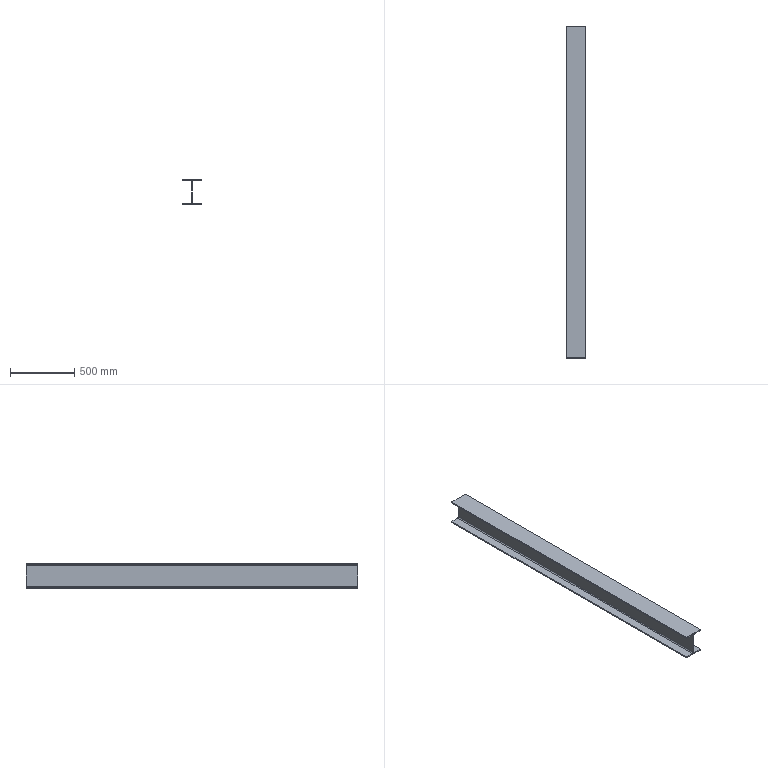Part | STEP file | Metering column 5 body_Default<As Machined> | 1 solid | 18 faces | box 150 x 2578 x 194 mm | volume 9824598 mm3 | plane 14 | cylinder 4 | commonest cylinder face diameters 16 x4
STEP:
#1=CARTESIAN_POINT('',(0.,0.,0.));
#2=DIRECTION('',(0.,0.,1.));
#3=DIRECTION('',(1.,0.,0.));
#4=AXIS2_PLACEMENT_3D('',#1,#2,#3);
#5=CARTESIAN_POINT('',(75.,0.,-88.));
#6=VERTEX_POINT('',#5);
#7=CARTESIAN_POINT('',(75.,0.,-97.));
#8=VERTEX_POINT('',#7);
#9=CARTESIAN_POINT('',(75.,0.,-97.));
#10=DIRECTION('',(0.,0.,-1.));
#11=VECTOR('',#10,1.);
#12=LINE('',#9,#11);
#13=CARTESIAN_POINT('',(75.,2578.,-97.));
#14=DIRECTION('',(-1.,0.,0.));
#15=DIRECTION('',(0.,0.,1.));
#16=AXIS2_PLACEMENT_3D('',#13,#14,#15);
#17=PLANE('',#16);
#18=CARTESIAN_POINT('',(0.,-2578.));
#19=DIRECTION('',(-1.,0.));
#20=VECTOR('',#19,1.);
#21=LINE('',#18,#20);
#22=(GEOMETRIC_REPRESENTATION_CONTEXT(2)PARAMETRIC_REPRESENTATION_CONTEXT()REPRESENTATION_CONTEXT('',''));
#23=DEFINITIONAL_REPRESENTATION('',(#21),#22);
#24=PCURVE('',#17,#23);
#25=CARTESIAN_POINT('',(11.,0.,-80.));
#26=DIRECTION('',(0.,1.,0.));
#27=DIRECTION('',(0.,0.,1.));
#28=AXIS2_PLACEMENT_3D('',#25,#26,#27);
#29=PLANE('',#28);
#30=CARTESIAN_POINT('',(-17.,64.));
#31=DIRECTION('',(-1.,0.));
#32=VECTOR('',#31,1.);
#33=LINE('',#30,#32);
#34=(GEOMETRIC_REPRESENTATION_CONTEXT(2)PARAMETRIC_REPRESENTATION_CONTEXT()REPRESENTATION_CONTEXT('',''));
#35=DEFINITIONAL_REPRESENTATION('',(#33),#34);
#36=PCURVE('',#29,#35);
#37=SURFACE_CURVE('',#12,(#24,#36),.PCURVE_S1.);
#38=EDGE_CURVE('',#6,#8,#37,.T.);
#39=ORIENTED_EDGE('',*,*,#38,.T.);
#40=CARTESIAN_POINT('',(75.,2578.,-97.));
#41=VERTEX_POINT('',#40);
#42=CARTESIAN_POINT('',(75.,2578.,-97.));
#43=DIRECTION('',(0.,-1.,0.));
#44=VECTOR('',#43,1.);
#45=LINE('',#42,#44);
#46=CARTESIAN_POINT('',(0.,0.));
#47=DIRECTION('',(0.,-1.));
#48=VECTOR('',#47,1.);
#49=LINE('',#46,#48);
#50=(GEOMETRIC_REPRESENTATION_CONTEXT(2)PARAMETRIC_REPRESENTATION_CONTEXT()REPRESENTATION_CONTEXT('',''));
#51=DEFINITIONAL_REPRESENTATION('',(#49),#50);
#52=PCURVE('',#17,#51);
#53=CARTESIAN_POINT('',(75.,2578.,-97.));
#54=DIRECTION('',(0.,0.,1.));
#55=DIRECTION('',(1.,0.,0.));
#56=AXIS2_PLACEMENT_3D('',#53,#54,#55);
#57=PLANE('',#56);
#58=CARTESIAN_POINT('',(0.,0.));
#59=DIRECTION('',(0.,-1.));
#60=VECTOR('',#59,1.);
#61=LINE('',#58,#60);
#62=(GEOMETRIC_REPRESENTATION_CONTEXT(2)PARAMETRIC_REPRESENTATION_CONTEXT()REPRESENTATION_CONTEXT('',''));
#63=DEFINITIONAL_REPRESENTATION('',(#61),#62);
#64=PCURVE('',#57,#63);
#65=SURFACE_CURVE('',#45,(#52,#64),.PCURVE_S1.);
#66=EDGE_CURVE('',#41,#8,#65,.T.);
#67=ORIENTED_EDGE('',*,*,#66,.F.);
#68=CARTESIAN_POINT('',(75.,2578.,-88.));
#69=VERTEX_POINT('',#68);
#70=CARTESIAN_POINT('',(75.,2578.,-97.));
#71=DIRECTION('',(0.,0.,-1.));
#72=VECTOR('',#71,1.);
#73=LINE('',#70,#72);
#74=CARTESIAN_POINT('',(0.,0.));
#75=DIRECTION('',(-1.,0.));
#76=VECTOR('',#75,1.);
#77=LINE('',#74,#76);
#78=(GEOMETRIC_REPRESENTATION_CONTEXT(2)PARAMETRIC_REPRESENTATION_CONTEXT()REPRESENTATION_CONTEXT('',''));
#79=DEFINITIONAL_REPRESENTATION('',(#77),#78);
#80=PCURVE('',#17,#79);
#81=CARTESIAN_POINT('',(11.,2578.,-80.));
#82=DIRECTION('',(0.,1.,0.));
#83=DIRECTION('',(0.,0.,1.));
#84=AXIS2_PLACEMENT_3D('',#81,#82,#83);
#85=PLANE('',#84);
#86=CARTESIAN_POINT('',(-17.,64.));
#87=DIRECTION('',(-1.,0.));
#88=VECTOR('',#87,1.);
#89=LINE('',#86,#88);
#90=(GEOMETRIC_REPRESENTATION_CONTEXT(2)PARAMETRIC_REPRESENTATION_CONTEXT()REPRESENTATION_CONTEXT('',''));
#91=DEFINITIONAL_REPRESENTATION('',(#89),#90);
#92=PCURVE('',#85,#91);
#93=SURFACE_CURVE('',#73,(#80,#92),.PCURVE_S1.);
#94=EDGE_CURVE('',#69,#41,#93,.T.);
#95=ORIENTED_EDGE('',*,*,#94,.F.);
#96=CARTESIAN_POINT('',(75.,2578.,-88.));
#97=DIRECTION('',(0.,-1.,0.));
#98=VECTOR('',#97,1.);
#99=LINE('',#96,#98);
#100=CARTESIAN_POINT('',(9.,0.));
#101=DIRECTION('',(0.,-1.));
#102=VECTOR('',#101,1.);
#103=LINE('',#100,#102);
#104=(GEOMETRIC_REPRESENTATION_CONTEXT(2)PARAMETRIC_REPRESENTATION_CONTEXT()REPRESENTATION_CONTEXT('',''));
#105=DEFINITIONAL_REPRESENTATION('',(#103),#104);
#106=PCURVE('',#17,#105);
#107=CARTESIAN_POINT('',(75.,2578.,-88.));
#108=DIRECTION('',(0.,0.,-1.));
#109=DIRECTION('',(-1.,0.,0.));
#110=AXIS2_PLACEMENT_3D('',#107,#108,#109);
#111=PLANE('',#110);
#112=CARTESIAN_POINT('',(0.,0.));
#113=DIRECTION('',(0.,-1.));
#114=VECTOR('',#113,1.);
#115=LINE('',#112,#114);
#116=(GEOMETRIC_REPRESENTATION_CONTEXT(2)PARAMETRIC_REPRESENTATION_CONTEXT()REPRESENTATION_CONTEXT('',''));
#117=DEFINITIONAL_REPRESENTATION('',(#115),#116);
#118=PCURVE('',#111,#117);
#119=SURFACE_CURVE('',#99,(#106,#118),.PCURVE_S1.);
#120=EDGE_CURVE('',#69,#6,#119,.T.);
#121=ORIENTED_EDGE('',*,*,#120,.T.);
#122=EDGE_LOOP('',(#39,#67,#95,#121));
#123=FACE_BOUND('',#122,.T.);
#124=ADVANCED_FACE('',(#123),#17,.F.);
#125=CARTESIAN_POINT('',(-75.,0.,-97.));
#126=VERTEX_POINT('',#125);
#127=CARTESIAN_POINT('',(75.,0.,-97.));
#128=DIRECTION('',(-1.,0.,0.));
#129=VECTOR('',#128,1.);
#130=LINE('',#127,#129);
#131=CARTESIAN_POINT('',(0.,-2578.));
#132=DIRECTION('',(-1.,0.));
#133=VECTOR('',#132,1.);
#134=LINE('',#131,#133);
#135=(GEOMETRIC_REPRESENTATION_CONTEXT(2)PARAMETRIC_REPRESENTATION_CONTEXT()REPRESENTATION_CONTEXT('',''));
#136=DEFINITIONAL_REPRESENTATION('',(#134),#135);
#137=PCURVE('',#57,#136);
#138=CARTESIAN_POINT('',(-17.,64.));
#139=DIRECTION('',(0.,-1.));
#140=VECTOR('',#139,1.);
#141=LINE('',#138,#140);
#142=(GEOMETRIC_REPRESENTATION_CONTEXT(2)PARAMETRIC_REPRESENTATION_CONTEXT()REPRESENTATION_CONTEXT('',''));
#143=DEFINITIONAL_REPRESENTATION('',(#141),#142);
#144=PCURVE('',#29,#143);
#145=SURFACE_CURVE('',#130,(#137,#144),.PCURVE_S1.);
#146=EDGE_CURVE('',#8,#126,#145,.T.);
#147=ORIENTED_EDGE('',*,*,#146,.T.);
#148=CARTESIAN_POINT('',(-75.,2578.,-97.));
#149=VERTEX_POINT('',#148);
#150=CARTESIAN_POINT('',(-75.,2578.,-97.));
#151=DIRECTION('',(0.,-1.,0.));
#152=VECTOR('',#151,1.);
#153=LINE('',#150,#152);
#154=CARTESIAN_POINT('',(-150.,0.));
#155=DIRECTION('',(0.,-1.));
#156=VECTOR('',#155,1.);
#157=LINE('',#154,#156);
#158=(GEOMETRIC_REPRESENTATION_CONTEXT(2)PARAMETRIC_REPRESENTATION_CONTEXT()REPRESENTATION_CONTEXT('',''));
#159=DEFINITIONAL_REPRESENTATION('',(#157),#158);
#160=PCURVE('',#57,#159);
#161=CARTESIAN_POINT('',(-75.,2578.,-88.));
#162=DIRECTION('',(1.,0.,0.));
#163=DIRECTION('',(0.,0.,-1.));
#164=AXIS2_PLACEMENT_3D('',#161,#162,#163);
#165=PLANE('',#164);
#166=CARTESIAN_POINT('',(9.,0.));
#167=DIRECTION('',(0.,-1.));
#168=VECTOR('',#167,1.);
#169=LINE('',#166,#168);
#170=(GEOMETRIC_REPRESENTATION_CONTEXT(2)PARAMETRIC_REPRESENTATION_CONTEXT()REPRESENTATION_CONTEXT('',''));
#171=DEFINITIONAL_REPRESENTATION('',(#169),#170);
#172=PCURVE('',#165,#171);
#173=SURFACE_CURVE('',#153,(#160,#172),.PCURVE_S1.);
#174=EDGE_CURVE('',#149,#126,#173,.T.);
#175=ORIENTED_EDGE('',*,*,#174,.F.);
#176=CARTESIAN_POINT('',(75.,2578.,-97.));
#177=DIRECTION('',(-1.,0.,0.));
#178=VECTOR('',#177,1.);
#179=LINE('',#176,#178);
#180=CARTESIAN_POINT('',(0.,0.));
#181=DIRECTION('',(-1.,0.));
#182=VECTOR('',#181,1.);
#183=LINE('',#180,#182);
#184=(GEOMETRIC_REPRESENTATION_CONTEXT(2)PARAMETRIC_REPRESENTATION_CONTEXT()REPRESENTATION_CONTEXT('',''));
#185=DEFINITIONAL_REPRESENTATION('',(#183),#184);
#186=PCURVE('',#57,#185);
#187=CARTESIAN_POINT('',(-17.,64.));
#188=DIRECTION('',(0.,-1.));
#189=VECTOR('',#188,1.);
#190=LINE('',#187,#189);
#191=(GEOMETRIC_REPRESENTATION_CONTEXT(2)PARAMETRIC_REPRESENTATION_CONTEXT()REPRESENTATION_CONTEXT('',''));
#192=DEFINITIONAL_REPRESENTATION('',(#190),#191);
#193=PCURVE('',#85,#192);
#194=SURFACE_CURVE('',#179,(#186,#193),.PCURVE_S1.);
#195=EDGE_CURVE('',#41,#149,#194,.T.);
#196=ORIENTED_EDGE('',*,*,#195,.F.);
#197=ORIENTED_EDGE('',*,*,#66,.T.);
#198=EDGE_LOOP('',(#147,#175,#196,#197));
#199=FACE_BOUND('',#198,.T.);
#200=ADVANCED_FACE('',(#199),#57,.F.);
#201=CARTESIAN_POINT('',(-75.,0.,-88.));
#202=VERTEX_POINT('',#201);
#203=CARTESIAN_POINT('',(-75.,0.,-88.));
#204=DIRECTION('',(0.,0.,1.));
#205=VECTOR('',#204,1.);
#206=LINE('',#203,#205);
#207=CARTESIAN_POINT('',(0.,-2578.));
#208=DIRECTION('',(-1.,0.));
#209=VECTOR('',#208,1.);
#210=LINE('',#207,#209);
#211=(GEOMETRIC_REPRESENTATION_CONTEXT(2)PARAMETRIC_REPRESENTATION_CONTEXT()REPRESENTATION_CONTEXT('',''));
#212=DEFINITIONAL_REPRESENTATION('',(#210),#211);
#213=PCURVE('',#165,#212);
#214=CARTESIAN_POINT('',(-8.,-86.));
#215=DIRECTION('',(1.,0.));
#216=VECTOR('',#215,1.);
#217=LINE('',#214,#216);
#218=(GEOMETRIC_REPRESENTATION_CONTEXT(2)PARAMETRIC_REPRESENTATION_CONTEXT()REPRESENTATION_CONTEXT('',''));
#219=DEFINITIONAL_REPRESENTATION('',(#217),#218);
#220=PCURVE('',#29,#219);
#221=SURFACE_CURVE('',#206,(#213,#220),.PCURVE_S1.);
#222=EDGE_CURVE('',#126,#202,#221,.T.);
#223=ORIENTED_EDGE('',*,*,#222,.T.);
#224=CARTESIAN_POINT('',(-75.,2578.,-88.));
#225=VERTEX_POINT('',#224);
#226=CARTESIAN_POINT('',(-75.,2578.,-88.));
#227=DIRECTION('',(0.,-1.,0.));
#228=VECTOR('',#227,1.);
#229=LINE('',#226,#228);
#230=CARTESIAN_POINT('',(0.,0.));
#231=DIRECTION('',(0.,-1.));
#232=VECTOR('',#231,1.);
#233=LINE('',#230,#232);
#234=(GEOMETRIC_REPRESENTATION_CONTEXT(2)PARAMETRIC_REPRESENTATION_CONTEXT()REPRESENTATION_CONTEXT('',''));
#235=DEFINITIONAL_REPRESENTATION('',(#233),#234);
#236=PCURVE('',#165,#235);
#237=CARTESIAN_POINT('',(-11.,2578.,-88.));
#238=DIRECTION('',(0.,0.,-1.));
#239=DIRECTION('',(-1.,0.,0.));
#240=AXIS2_PLACEMENT_3D('',#237,#238,#239);
#241=PLANE('',#240);
#242=CARTESIAN_POINT('',(64.,0.));
#243=DIRECTION('',(0.,-1.));
#244=VECTOR('',#243,1.);
#245=LINE('',#242,#244);
#246=(GEOMETRIC_REPRESENTATION_CONTEXT(2)PARAMETRIC_REPRESENTATION_CONTEXT()REPRESENTATION_CONTEXT('',''));
#247=DEFINITIONAL_REPRESENTATION('',(#245),#246);
#248=PCURVE('',#241,#247);
#249=SURFACE_CURVE('',#229,(#236,#248),.PCURVE_S1.);
#250=EDGE_CURVE('',#225,#202,#249,.T.);
#251=ORIENTED_EDGE('',*,*,#250,.F.);
#252=CARTESIAN_POINT('',(-75.,2578.,-88.));
#253=DIRECTION('',(0.,0.,1.));
#254=VECTOR('',#253,1.);
#255=LINE('',#252,#254);
#256=CARTESIAN_POINT('',(0.,0.));
#257=DIRECTION('',(-1.,0.));
#258=VECTOR('',#257,1.);
#259=LINE('',#256,#258);
#260=(GEOMETRIC_REPRESENTATION_CONTEXT(2)PARAMETRIC_REPRESENTATION_CONTEXT()REPRESENTATION_CONTEXT('',''));
#261=DEFINITIONAL_REPRESENTATION('',(#259),#260);
#262=PCURVE('',#165,#261);
#263=CARTESIAN_POINT('',(-8.,-86.));
#264=DIRECTION('',(1.,0.));
#265=VECTOR('',#264,1.);
#266=LINE('',#263,#265);
#267=(GEOMETRIC_REPRESENTATION_CONTEXT(2)PARAMETRIC_REPRESENTATION_CONTEXT()REPRESENTATION_CONTEXT('',''));
#268=DEFINITIONAL_REPRESENTATION('',(#266),#267);
#269=PCURVE('',#85,#268);
#270=SURFACE_CURVE('',#255,(#262,#269),.PCURVE_S1.);
#271=EDGE_CURVE('',#149,#225,#270,.T.);
#272=ORIENTED_EDGE('',*,*,#271,.F.);
#273=ORIENTED_EDGE('',*,*,#174,.T.);
#274=EDGE_LOOP('',(#223,#251,#272,#273));
#275=FACE_BOUND('',#274,.T.);
#276=ADVANCED_FACE('',(#275),#165,.F.);
#277=CARTESIAN_POINT('',(-11.,0.,-88.));
#278=VERTEX_POINT('',#277);
#279=CARTESIAN_POINT('',(-11.,0.,-88.));
#280=DIRECTION('',(1.,0.,0.));
#281=VECTOR('',#280,1.);
#282=LINE('',#279,#281);
#283=CARTESIAN_POINT('',(0.,-2578.));
#284=DIRECTION('',(-1.,0.));
#285=VECTOR('',#284,1.);
#286=LINE('',#283,#285);
#287=(GEOMETRIC_REPRESENTATION_CONTEXT(2)PARAMETRIC_REPRESENTATION_CONTEXT()REPRESENTATION_CONTEXT('',''));
#288=DEFINITIONAL_REPRESENTATION('',(#286),#287);
#289=PCURVE('',#241,#288);
#290=CARTESIAN_POINT('',(-8.,-22.));
#291=DIRECTION('',(0.,1.));
#292=VECTOR('',#291,1.);
#293=LINE('',#290,#292);
#294=(GEOMETRIC_REPRESENTATION_CONTEXT(2)PARAMETRIC_REPRESENTATION_CONTEXT()REPRESENTATION_CONTEXT('',''));
#295=DEFINITIONAL_REPRESENTATION('',(#293),#294);
#296=PCURVE('',#29,#295);
#297=SURFACE_CURVE('',#282,(#289,#296),.PCURVE_S1.);
#298=EDGE_CURVE('',#202,#278,#297,.T.);
#299=ORIENTED_EDGE('',*,*,#298,.T.);
#300=CARTESIAN_POINT('',(-11.,2578.,-88.));
#301=VERTEX_POINT('',#300);
#302=CARTESIAN_POINT('',(-11.,2578.,-88.));
#303=DIRECTION('',(0.,-1.,0.));
#304=VECTOR('',#303,1.);
#305=LINE('',#302,#304);
#306=CARTESIAN_POINT('',(0.,0.));
#307=DIRECTION('',(0.,-1.));
#308=VECTOR('',#307,1.);
#309=LINE('',#306,#308);
#310=(GEOMETRIC_REPRESENTATION_CONTEXT(2)PARAMETRIC_REPRESENTATION_CONTEXT()REPRESENTATION_CONTEXT('',''));
#311=DEFINITIONAL_REPRESENTATION('',(#309),#310);
#312=PCURVE('',#241,#311);
#313=CARTESIAN_POINT('',(-11.,2578.,-80.));
#314=DIRECTION('',(0.,-1.,0.));
#315=DIRECTION('',(0.,0.,-1.));
#316=AXIS2_PLACEMENT_3D('',#313,#314,#315);
#317=CYLINDRICAL_SURFACE('',#316,8.);
#318=CARTESIAN_POINT('',(0.,0.));
#319=DIRECTION('',(0.,1.));
#320=VECTOR('',#319,1.);
#321=LINE('',#318,#320);
#322=(GEOMETRIC_REPRESENTATION_CONTEXT(2)PARAMETRIC_REPRESENTATION_CONTEXT()REPRESENTATION_CONTEXT('',''));
#323=DEFINITIONAL_REPRESENTATION('',(#321),#322);
#324=PCURVE('',#317,#323);
#325=SURFACE_CURVE('',#305,(#312,#324),.PCURVE_S1.);
#326=EDGE_CURVE('',#301,#278,#325,.T.);
#327=ORIENTED_EDGE('',*,*,#326,.F.);
#328=CARTESIAN_POINT('',(-11.,2578.,-88.));
#329=DIRECTION('',(1.,0.,0.));
#330=VECTOR('',#329,1.);
#331=LINE('',#328,#330);
#332=CARTESIAN_POINT('',(0.,0.));
#333=DIRECTION('',(-1.,0.));
#334=VECTOR('',#333,1.);
#335=LINE('',#332,#334);
#336=(GEOMETRIC_REPRESENTATION_CONTEXT(2)PARAMETRIC_REPRESENTATION_CONTEXT()REPRESENTATION_CONTEXT('',''));
#337=DEFINITIONAL_REPRESENTATION('',(#335),#336);
#338=PCURVE('',#241,#337);
#339=CARTESIAN_POINT('',(-8.,-22.));
#340=DIRECTION('',(0.,1.));
#341=VECTOR('',#340,1.);
#342=LINE('',#339,#341);
#343=(GEOMETRIC_REPRESENTATION_CONTEXT(2)PARAMETRIC_REPRESENTATION_CONTEXT()REPRESENTATION_CONTEXT('',''));
#344=DEFINITIONAL_REPRESENTATION('',(#342),#343);
#345=PCURVE('',#85,#344);
#346=SURFACE_CURVE('',#331,(#338,#345),.PCURVE_S1.);
#347=EDGE_CURVE('',#225,#301,#346,.T.);
#348=ORIENTED_EDGE('',*,*,#347,.F.);
#349=ORIENTED_EDGE('',*,*,#250,.T.);
#350=EDGE_LOOP('',(#299,#327,#348,#349));
#351=FACE_BOUND('',#350,.T.);
#352=ADVANCED_FACE('',(#351),#241,.F.);
#353=ORIENTED_EDGE('',*,*,#326,.F.);
#354=CARTESIAN_POINT('',(-3.,2578.,-80.));
#355=VERTEX_POINT('',#354);
#356=CARTESIAN_POINT('',(-11.,2578.,-80.));
#357=DIRECTION('',(0.,-1.,0.));
#358=DIRECTION('',(0.,0.,1.));
#359=AXIS2_PLACEMENT_3D('',#356,#357,#358);
#360=CIRCLE('',#359,8.);
#361=CARTESIAN_POINT('',(-3.142,0.));
#362=DIRECTION('',(1.,0.));
#363=VECTOR('',#362,1.);
#364=LINE('',#361,#363);
#365=(GEOMETRIC_REPRESENTATION_CONTEXT(2)PARAMETRIC_REPRESENTATION_CONTEXT()REPRESENTATION_CONTEXT('',''));
#366=DEFINITIONAL_REPRESENTATION('',(#364),#365);
#367=PCURVE('',#317,#366);
#368=CARTESIAN_POINT('',(8.,-22.));
#369=CARTESIAN_POINT('',(8.,-35.856));
#370=CARTESIAN_POINT('',(-4.,-28.928));
#371=CARTESIAN_POINT('',(-16.,-22.));
#372=CARTESIAN_POINT('',(-4.,-15.072));
#373=CARTESIAN_POINT('',(8.,-8.144));
#374=CARTESIAN_POINT('',(8.,-22.));
#375=(BOUNDED_CURVE()B_SPLINE_CURVE(2,(#368,#369,#370,#371,#372,#373,#374),.UNSPECIFIED.,.T.,.F.)B_SPLINE_CURVE_WITH_KNOTS((1,2,2,2,2,1),(-2.094,0.,2.094,4.189,6.283,8.378),.UNSPECIFIED.)CURVE()GEOMETRIC_REPRESENTATION_ITEM()RATIONAL_B_SPLINE_CURVE((1.,0.5,1.,0.5,1.,0.5,1.))REPRESENTATION_ITEM(''));
#376=(GEOMETRIC_REPRESENTATION_CONTEXT(2)PARAMETRIC_REPRESENTATION_CONTEXT()REPRESENTATION_CONTEXT('',''));
#377=DEFINITIONAL_REPRESENTATION('',(#375),#376);
#378=PCURVE('',#85,#377);
#379=SURFACE_CURVE('',#360,(#367,#378),.PCURVE_S1.);
#380=EDGE_CURVE('',#301,#355,#379,.T.);
#381=ORIENTED_EDGE('',*,*,#380,.T.);
#382=CARTESIAN_POINT('',(-3.,0.,-80.));
#383=VERTEX_POINT('',#382);
#384=CARTESIAN_POINT('',(-3.,2578.,-80.));
#385=DIRECTION('',(0.,-1.,0.));
#386=VECTOR('',#385,1.);
#387=LINE('',#384,#386);
#388=CARTESIAN_POINT('',(1.571,0.));
#389=DIRECTION('',(0.,1.));
#390=VECTOR('',#389,1.);
#391=LINE('',#388,#390);
#392=(GEOMETRIC_REPRESENTATION_CONTEXT(2)PARAMETRIC_REPRESENTATION_CONTEXT()REPRESENTATION_CONTEXT('',''));
#393=DEFINITIONAL_REPRESENTATION('',(#391),#392);
#394=PCURVE('',#317,#393);
#395=CARTESIAN_POINT('',(-3.,2578.,80.));
#396=DIRECTION('',(1.,0.,0.));
#397=DIRECTION('',(0.,0.,-1.));
#398=AXIS2_PLACEMENT_3D('',#395,#396,#397);
#399=PLANE('',#398);
#400=CARTESIAN_POINT('',(160.,0.));
#401=DIRECTION('',(0.,-1.));
#402=VECTOR('',#401,1.);
#403=LINE('',#400,#402);
#404=(GEOMETRIC_REPRESENTATION_CONTEXT(2)PARAMETRIC_REPRESENTATION_CONTEXT()REPRESENTATION_CONTEXT('',''));
#405=DEFINITIONAL_REPRESENTATION('',(#403),#404);
#406=PCURVE('',#399,#405);
#407=SURFACE_CURVE('',#387,(#394,#406),.PCURVE_S1.);
#408=EDGE_CURVE('',#355,#383,#407,.T.);
#409=ORIENTED_EDGE('',*,*,#408,.T.);
#410=CARTESIAN_POINT('',(-11.,0.,-80.));
#411=DIRECTION('',(0.,-1.,0.));
#412=DIRECTION('',(0.,0.,1.));
#413=AXIS2_PLACEMENT_3D('',#410,#411,#412);
#414=CIRCLE('',#413,8.);
#415=CARTESIAN_POINT('',(-3.142,2578.));
#416=DIRECTION('',(1.,0.));
#417=VECTOR('',#416,1.);
#418=LINE('',#415,#417);
#419=(GEOMETRIC_REPRESENTATION_CONTEXT(2)PARAMETRIC_REPRESENTATION_CONTEXT()REPRESENTATION_CONTEXT('',''));
#420=DEFINITIONAL_REPRESENTATION('',(#418),#419);
#421=PCURVE('',#317,#420);
#422=CARTESIAN_POINT('',(8.,-22.));
#423=CARTESIAN_POINT('',(8.,-35.856));
#424=CARTESIAN_POINT('',(-4.,-28.928));
#425=CARTESIAN_POINT('',(-16.,-22.));
#426=CARTESIAN_POINT('',(-4.,-15.072));
#427=CARTESIAN_POINT('',(8.,-8.144));
#428=CARTESIAN_POINT('',(8.,-22.));
#429=(BOUNDED_CURVE()B_SPLINE_CURVE(2,(#422,#423,#424,#425,#426,#427,#428),.UNSPECIFIED.,.T.,.F.)B_SPLINE_CURVE_WITH_KNOTS((1,2,2,2,2,1),(-2.094,0.,2.094,4.189,6.283,8.378),.UNSPECIFIED.)CURVE()GEOMETRIC_REPRESENTATION_ITEM()RATIONAL_B_SPLINE_CURVE((1.,0.5,1.,0.5,1.,0.5,1.))REPRESENTATION_ITEM(''));
#430=(GEOMETRIC_REPRESENTATION_CONTEXT(2)PARAMETRIC_REPRESENTATION_CONTEXT()REPRESENTATION_CONTEXT('',''));
#431=DEFINITIONAL_REPRESENTATION('',(#429),#430);
#432=PCURVE('',#29,#431);
#433=SURFACE_CURVE('',#414,(#421,#432),.PCURVE_S1.);
#434=EDGE_CURVE('',#278,#383,#433,.T.);
#435=ORIENTED_EDGE('',*,*,#434,.F.);
#436=EDGE_LOOP('',(#353,#381,#409,#435));
#437=FACE_BOUND('',#436,.F.);
#438=ADVANCED_FACE('',(#437),#317,.F.);
#439=CARTESIAN_POINT('',(-3.,0.,80.));
#440=VERTEX_POINT('',#439);
#441=CARTESIAN_POINT('',(-3.,0.,80.));
#442=DIRECTION('',(0.,0.,1.));
#443=VECTOR('',#442,1.);
#444=LINE('',#441,#443);
#445=CARTESIAN_POINT('',(0.,-2578.));
#446=DIRECTION('',(-1.,0.));
#447=VECTOR('',#446,1.);
#448=LINE('',#445,#447);
#449=(GEOMETRIC_REPRESENTATION_CONTEXT(2)PARAMETRIC_REPRESENTATION_CONTEXT()REPRESENTATION_CONTEXT('',''));
#450=DEFINITIONAL_REPRESENTATION('',(#448),#449);
#451=PCURVE('',#399,#450);
#452=CARTESIAN_POINT('',(160.,-14.));
#453=DIRECTION('',(1.,0.));
#454=VECTOR('',#453,1.);
#455=LINE('',#452,#454);
#456=(GEOMETRIC_REPRESENTATION_CONTEXT(2)PARAMETRIC_REPRESENTATION_CONTEXT()REPRESENTATION_CONTEXT('',''));
#457=DEFINITIONAL_REPRESENTATION('',(#455),#456);
#458=PCURVE('',#29,#457);
#459=SURFACE_CURVE('',#444,(#451,#458),.PCURVE_S1.);
#460=EDGE_CURVE('',#383,#440,#459,.T.);
#461=ORIENTED_EDGE('',*,*,#460,.T.);
#462=CARTESIAN_POINT('',(-3.,2578.,80.));
#463=VERTEX_POINT('',#462);
#464=CARTESIAN_POINT('',(-3.,2578.,80.));
#465=DIRECTION('',(0.,-1.,0.));
#466=VECTOR('',#465,1.);
#467=LINE('',#464,#466);
#468=CARTESIAN_POINT('',(0.,0.));
#469=DIRECTION('',(0.,-1.));
#470=VECTOR('',#469,1.);
#471=LINE('',#468,#470);
#472=(GEOMETRIC_REPRESENTATION_CONTEXT(2)PARAMETRIC_REPRESENTATION_CONTEXT()REPRESENTATION_CONTEXT('',''));
#473=DEFINITIONAL_REPRESENTATION('',(#471),#472);
#474=PCURVE('',#399,#473);
#475=CARTESIAN_POINT('',(-11.,2578.,80.));
#476=DIRECTION('',(0.,-1.,0.));
#477=DIRECTION('',(0.,0.,-1.));
#478=AXIS2_PLACEMENT_3D('',#475,#476,#477);
#479=CYLINDRICAL_SURFACE('',#478,8.);
#480=CARTESIAN_POINT('',(1.571,0.));
#481=DIRECTION('',(0.,1.));
#482=VECTOR('',#481,1.);
#483=LINE('',#480,#482);
#484=(GEOMETRIC_REPRESENTATION_CONTEXT(2)PARAMETRIC_REPRESENTATION_CONTEXT()REPRESENTATION_CONTEXT('',''));
#485=DEFINITIONAL_REPRESENTATION('',(#483),#484);
#486=PCURVE('',#479,#485);
#487=SURFACE_CURVE('',#467,(#474,#486),.PCURVE_S1.);
#488=EDGE_CURVE('',#463,#440,#487,.T.);
#489=ORIENTED_EDGE('',*,*,#488,.F.);
#490=CARTESIAN_POINT('',(-3.,2578.,80.));
#491=DIRECTION('',(0.,0.,1.));
#492=VECTOR('',#491,1.);
#493=LINE('',#490,#492);
#494=CARTESIAN_POINT('',(0.,0.));
#495=DIRECTION('',(-1.,0.));
#496=VECTOR('',#495,1.);
#497=LINE('',#494,#496);
#498=(GEOMETRIC_REPRESENTATION_CONTEXT(2)PARAMETRIC_REPRESENTATION_CONTEXT()REPRESENTATION_CONTEXT('',''));
#499=DEFINITIONAL_REPRESENTATION('',(#497),#498);
#500=PCURVE('',#399,#499);
#501=CARTESIAN_POINT('',(160.,-14.));
#502=DIRECTION('',(1.,0.));
#503=VECTOR('',#502,1.);
#504=LINE('',#501,#503);
#505=(GEOMETRIC_REPRESENTATION_CONTEXT(2)PARAMETRIC_REPRESENTATION_CONTEXT()REPRESENTATION_CONTEXT('',''));
#506=DEFINITIONAL_REPRESENTATION('',(#504),#505);
#507=PCURVE('',#85,#506);
#508=SURFACE_CURVE('',#493,(#500,#507),.PCURVE_S1.);
#509=EDGE_CURVE('',#355,#463,#508,.T.);
#510=ORIENTED_EDGE('',*,*,#509,.F.);
#511=ORIENTED_EDGE('',*,*,#408,.T.);
#512=EDGE_LOOP('',(#461,#489,#510,#511));
#513=FACE_BOUND('',#512,.T.);
#514=ADVANCED_FACE('',(#513),#399,.F.);
#515=ORIENTED_EDGE('',*,*,#488,.F.);
#516=CARTESIAN_POINT('',(-11.,2578.,88.));
#517=VERTEX_POINT('',#516);
#518=CARTESIAN_POINT('',(-11.,2578.,80.));
#519=DIRECTION('',(0.,-1.,0.));
#520=DIRECTION('',(0.,0.,1.));
#521=AXIS2_PLACEMENT_3D('',#518,#519,#520);
#522=CIRCLE('',#521,8.);
#523=CARTESIAN_POINT('',(-3.142,0.));
#524=DIRECTION('',(1.,0.));
#525=VECTOR('',#524,1.);
#526=LINE('',#523,#525);
#527=(GEOMETRIC_REPRESENTATION_CONTEXT(2)PARAMETRIC_REPRESENTATION_CONTEXT()REPRESENTATION_CONTEXT('',''));
#528=DEFINITIONAL_REPRESENTATION('',(#526),#527);
#529=PCURVE('',#479,#528);
#530=CARTESIAN_POINT('',(168.,-22.));
#531=CARTESIAN_POINT('',(168.,-35.856));
#532=CARTESIAN_POINT('',(156.,-28.928));
#533=CARTESIAN_POINT('',(144.,-22.));
#534=CARTESIAN_POINT('',(156.,-15.072));
#535=CARTESIAN_POINT('',(168.,-8.144));
#536=CARTESIAN_POINT('',(168.,-22.));
#537=(BOUNDED_CURVE()B_SPLINE_CURVE(2,(#530,#531,#532,#533,#534,#535,#536),.UNSPECIFIED.,.T.,.F.)B_SPLINE_CURVE_WITH_KNOTS((1,2,2,2,2,1),(-2.094,0.,2.094,4.189,6.283,8.378),.UNSPECIFIED.)CURVE()GEOMETRIC_REPRESENTATION_ITEM()RATIONAL_B_SPLINE_CURVE((1.,0.5,1.,0.5,1.,0.5,1.))REPRESENTATION_ITEM(''));
#538=(GEOMETRIC_REPRESENTATION_CONTEXT(2)PARAMETRIC_REPRESENTATION_CONTEXT()REPRESENTATION_CONTEXT('',''));
#539=DEFINITIONAL_REPRESENTATION('',(#537),#538);
#540=PCURVE('',#85,#539);
#541=SURFACE_CURVE('',#522,(#529,#540),.PCURVE_S1.);
#542=EDGE_CURVE('',#463,#517,#541,.T.);
#543=ORIENTED_EDGE('',*,*,#542,.T.);
#544=CARTESIAN_POINT('',(-11.,0.,88.));
#545=VERTEX_POINT('',#544);
#546=CARTESIAN_POINT('',(-11.,2578.,88.));
#547=DIRECTION('',(0.,-1.,0.));
#548=VECTOR('',#547,1.);
#549=LINE('',#546,#548);
#550=CARTESIAN_POINT('',(3.142,0.));
#551=DIRECTION('',(0.,1.));
#552=VECTOR('',#551,1.);
#553=LINE('',#550,#552);
#554=(GEOMETRIC_REPRESENTATION_CONTEXT(2)PARAMETRIC_REPRESENTATION_CONTEXT()REPRESENTATION_CONTEXT('',''));
#555=DEFINITIONAL_REPRESENTATION('',(#553),#554);
#556=PCURVE('',#479,#555);
#557=CARTESIAN_POINT('',(-75.,2578.,88.));
#558=DIRECTION('',(0.,0.,1.));
#559=DIRECTION('',(1.,0.,0.));
#560=AXIS2_PLACEMENT_3D('',#557,#558,#559);
#561=PLANE('',#560);
#562=CARTESIAN_POINT('',(64.,0.));
#563=DIRECTION('',(0.,-1.));
#564=VECTOR('',#563,1.);
#565=LINE('',#562,#564);
#566=(GEOMETRIC_REPRESENTATION_CONTEXT(2)PARAMETRIC_REPRESENTATION_CONTEXT()REPRESENTATION_CONTEXT('',''));
#567=DEFINITIONAL_REPRESENTATION('',(#565),#566);
#568=PCURVE('',#561,#567);
#569=SURFACE_CURVE('',#549,(#556,#568),.PCURVE_S1.);
#570=EDGE_CURVE('',#517,#545,#569,.T.);
#571=ORIENTED_EDGE('',*,*,#570,.T.);
#572=CARTESIAN_POINT('',(-11.,0.,80.));
#573=DIRECTION('',(0.,-1.,0.));
#574=DIRECTION('',(0.,0.,1.));
#575=AXIS2_PLACEMENT_3D('',#572,#573,#574);
#576=CIRCLE('',#575,8.);
#577=CARTESIAN_POINT('',(-3.142,2578.));
#578=DIRECTION('',(1.,0.));
#579=VECTOR('',#578,1.);
#580=LINE('',#577,#579);
#581=(GEOMETRIC_REPRESENTATION_CONTEXT(2)PARAMETRIC_REPRESENTATION_CONTEXT()REPRESENTATION_CONTEXT('',''));
#582=DEFINITIONAL_REPRESENTATION('',(#580),#581);
#583=PCURVE('',#479,#582);
#584=CARTESIAN_POINT('',(168.,-22.));
#585=CARTESIAN_POINT('',(168.,-35.856));
#586=CARTESIAN_POINT('',(156.,-28.928));
#587=CARTESIAN_POINT('',(144.,-22.));
#588=CARTESIAN_POINT('',(156.,-15.072));
#589=CARTESIAN_POINT('',(168.,-8.144));
#590=CARTESIAN_POINT('',(168.,-22.));
#591=(BOUNDED_CURVE()B_SPLINE_CURVE(2,(#584,#585,#586,#587,#588,#589,#590),.UNSPECIFIED.,.T.,.F.)B_SPLINE_CURVE_WITH_KNOTS((1,2,2,2,2,1),(-2.094,0.,2.094,4.189,6.283,8.378),.UNSPECIFIED.)CURVE()GEOMETRIC_REPRESENTATION_ITEM()RATIONAL_B_SPLINE_CURVE((1.,0.5,1.,0.5,1.,0.5,1.))REPRESENTATION_ITEM(''));
#592=(GEOMETRIC_REPRESENTATION_CONTEXT(2)PARAMETRIC_REPRESENTATION_CONTEXT()REPRESENTATION_CONTEXT('',''));
#593=DEFINITIONAL_REPRESENTATION('',(#591),#592);
#594=PCURVE('',#29,#593);
#595=SURFACE_CURVE('',#576,(#583,#594),.PCURVE_S1.);
#596=EDGE_CURVE('',#440,#545,#595,.T.);
#597=ORIENTED_EDGE('',*,*,#596,.F.);
#598=EDGE_LOOP('',(#515,#543,#571,#597));
#599=FACE_BOUND('',#598,.F.);
#600=ADVANCED_FACE('',(#599),#479,.F.);
#601=CARTESIAN_POINT('',(-75.,0.,88.));
#602=VERTEX_POINT('',#601);
#603=CARTESIAN_POINT('',(-75.,0.,88.));
#604=DIRECTION('',(-1.,0.,0.));
#605=VECTOR('',#604,1.);
#606=LINE('',#603,#605);
#607=CARTESIAN_POINT('',(0.,-2578.));
#608=DIRECTION('',(-1.,0.));
#609=VECTOR('',#608,1.);
#610=LINE('',#607,#609);
#611=(GEOMETRIC_REPRESENTATION_CONTEXT(2)PARAMETRIC_REPRESENTATION_CONTEXT()REPRESENTATION_CONTEXT('',''));
#612=DEFINITIONAL_REPRESENTATION('',(#610),#611);
#613=PCURVE('',#561,#612);
#614=CARTESIAN_POINT('',(168.,-86.));
#615=DIRECTION('',(0.,-1.));
#616=VECTOR('',#615,1.);
#617=LINE('',#614,#616);
#618=(GEOMETRIC_REPRESENTATION_CONTEXT(2)PARAMETRIC_REPRESENTATION_CONTEXT()REPRESENTATION_CONTEXT('',''));
#619=DEFINITIONAL_REPRESENTATION('',(#617),#618);
#620=PCURVE('',#29,#619);
#621=SURFACE_CURVE('',#606,(#613,#620),.PCURVE_S1.);
#622=EDGE_CURVE('',#545,#602,#621,.T.);
#623=ORIENTED_EDGE('',*,*,#622,.T.);
#624=CARTESIAN_POINT('',(-75.,2578.,88.));
#625=VERTEX_POINT('',#624);
#626=CARTESIAN_POINT('',(-75.,2578.,88.));
#627=DIRECTION('',(0.,-1.,0.));
#628=VECTOR('',#627,1.);
#629=LINE('',#626,#628);
#630=CARTESIAN_POINT('',(0.,0.));
#631=DIRECTION('',(0.,-1.));
#632=VECTOR('',#631,1.);
#633=LINE('',#630,#632);
#634=(GEOMETRIC_REPRESENTATION_CONTEXT(2)PARAMETRIC_REPRESENTATION_CONTEXT()REPRESENTATION_CONTEXT('',''));
#635=DEFINITIONAL_REPRESENTATION('',(#633),#634);
#636=PCURVE('',#561,#635);
#637=CARTESIAN_POINT('',(-75.,2578.,97.));
#638=DIRECTION('',(1.,0.,0.));
#639=DIRECTION('',(0.,0.,-1.));
#640=AXIS2_PLACEMENT_3D('',#637,#638,#639);
#641=PLANE('',#640);
#642=CARTESIAN_POINT('',(9.,0.));
#643=DIRECTION('',(0.,-1.));
#644=VECTOR('',#643,1.);
#645=LINE('',#642,#644);
#646=(GEOMETRIC_REPRESENTATION_CONTEXT(2)PARAMETRIC_REPRESENTATION_CONTEXT()REPRESENTATION_CONTEXT('',''));
#647=DEFINITIONAL_REPRESENTATION('',(#645),#646);
#648=PCURVE('',#641,#647);
#649=SURFACE_CURVE('',#629,(#636,#648),.PCURVE_S1.);
#650=EDGE_CURVE('',#625,#602,#649,.T.);
#651=ORIENTED_EDGE('',*,*,#650,.F.);
#652=CARTESIAN_POINT('',(-75.,2578.,88.));
#653=DIRECTION('',(-1.,0.,0.));
#654=VECTOR('',#653,1.);
#655=LINE('',#652,#654);
#656=CARTESIAN_POINT('',(0.,0.));
#657=DIRECTION('',(-1.,0.));
#658=VECTOR('',#657,1.);
#659=LINE('',#656,#658);
#660=(GEOMETRIC_REPRESENTATION_CONTEXT(2)PARAMETRIC_REPRESENTATION_CONTEXT()REPRESENTATION_CONTEXT('',''));
#661=DEFINITIONAL_REPRESENTATION('',(#659),#660);
#662=PCURVE('',#561,#661);
#663=CARTESIAN_POINT('',(168.,-86.));
#664=DIRECTION('',(0.,-1.));
#665=VECTOR('',#664,1.);
#666=LINE('',#663,#665);
#667=(GEOMETRIC_REPRESENTATION_CONTEXT(2)PARAMETRIC_REPRESENTATION_CONTEXT()REPRESENTATION_CONTEXT('',''));
#668=DEFINITIONAL_REPRESENTATION('',(#666),#667);
#669=PCURVE('',#85,#668);
#670=SURFACE_CURVE('',#655,(#662,#669),.PCURVE_S1.);
#671=EDGE_CURVE('',#517,#625,#670,.T.);
#672=ORIENTED_EDGE('',*,*,#671,.F.);
#673=ORIENTED_EDGE('',*,*,#570,.T.);
#674=EDGE_LOOP('',(#623,#651,#672,#673));
#675=FACE_BOUND('',#674,.T.);
#676=ADVANCED_FACE('',(#675),#561,.F.);
#677=CARTESIAN_POINT('',(-75.,0.,97.));
#678=VERTEX_POINT('',#677);
#679=CARTESIAN_POINT('',(-75.,0.,97.));
#680=DIRECTION('',(0.,0.,1.));
#681=VECTOR('',#680,1.);
#682=LINE('',#679,#681);
#683=CARTESIAN_POINT('',(0.,-2578.));
#684=DIRECTION('',(-1.,0.));
#685=VECTOR('',#684,1.);
#686=LINE('',#683,#685);
#687=(GEOMETRIC_REPRESENTATION_CONTEXT(2)PARAMETRIC_REPRESENTATION_CONTEXT()REPRESENTATION_CONTEXT('',''));
#688=DEFINITIONAL_REPRESENTATION('',(#686),#687);
#689=PCURVE('',#641,#688);
#690=CARTESIAN_POINT('',(177.,-86.));
#691=DIRECTION('',(1.,0.));
#692=VECTOR('',#691,1.);
#693=LINE('',#690,#692);
#694=(GEOMETRIC_REPRESENTATION_CONTEXT(2)PARAMETRIC_REPRESENTATION_CONTEXT()REPRESENTATION_CONTEXT('',''));
#695=DEFINITIONAL_REPRESENTATION('',(#693),#694);
#696=PCURVE('',#29,#695);
#697=SURFACE_CURVE('',#682,(#689,#696),.PCURVE_S1.);
#698=EDGE_CURVE('',#602,#678,#697,.T.);
#699=ORIENTED_EDGE('',*,*,#698,.T.);
#700=CARTESIAN_POINT('',(-75.,2578.,97.));
#701=VERTEX_POINT('',#700);
#702=CARTESIAN_POINT('',(-75.,2578.,97.));
#703=DIRECTION('',(0.,-1.,0.));
#704=VECTOR('',#703,1.);
#705=LINE('',#702,#704);
#706=CARTESIAN_POINT('',(0.,0.));
#707=DIRECTION('',(0.,-1.));
#708=VECTOR('',#707,1.);
#709=LINE('',#706,#708);
#710=(GEOMETRIC_REPRESENTATION_CONTEXT(2)PARAMETRIC_REPRESENTATION_CONTEXT()REPRESENTATION_CONTEXT('',''));
#711=DEFINITIONAL_REPRESENTATION('',(#709),#710);
#712=PCURVE('',#641,#711);
#713=CARTESIAN_POINT('',(75.,2578.,97.));
#714=DIRECTION('',(0.,0.,-1.));
#715=DIRECTION('',(-1.,0.,0.));
#716=AXIS2_PLACEMENT_3D('',#713,#714,#715);
#717=PLANE('',#716);
#718=CARTESIAN_POINT('',(150.,0.));
#719=DIRECTION('',(0.,-1.));
#720=VECTOR('',#719,1.);
#721=LINE('',#718,#720);
#722=(GEOMETRIC_REPRESENTATION_CONTEXT(2)PARAMETRIC_REPRESENTATION_CONTEXT()REPRESENTATION_CONTEXT('',''));
#723=DEFINITIONAL_REPRESENTATION('',(#721),#722);
#724=PCURVE('',#717,#723);
#725=SURFACE_CURVE('',#705,(#712,#724),.PCURVE_S1.);
#726=EDGE_CURVE('',#701,#678,#725,.T.);
#727=ORIENTED_EDGE('',*,*,#726,.F.);
#728=CARTESIAN_POINT('',(-75.,2578.,97.));
#729=DIRECTION('',(0.,0.,1.));
#730=VECTOR('',#729,1.);
#731=LINE('',#728,#730);
#732=CARTESIAN_POINT('',(0.,0.));
#733=DIRECTION('',(-1.,0.));
#734=VECTOR('',#733,1.);
#735=LINE('',#732,#734);
#736=(GEOMETRIC_REPRESENTATION_CONTEXT(2)PARAMETRIC_REPRESENTATION_CONTEXT()REPRESENTATION_CONTEXT('',''));
#737=DEFINITIONAL_REPRESENTATION('',(#735),#736);
#738=PCURVE('',#641,#737);
#739=CARTESIAN_POINT('',(177.,-86.));
#740=DIRECTION('',(1.,0.));
#741=VECTOR('',#740,1.);
#742=LINE('',#739,#741);
#743=(GEOMETRIC_REPRESENTATION_CONTEXT(2)PARAMETRIC_REPRESENTATION_CONTEXT()REPRESENTATION_CONTEXT('',''));
#744=DEFINITIONAL_REPRESENTATION('',(#742),#743);
#745=PCURVE('',#85,#744);
#746=SURFACE_CURVE('',#731,(#738,#745),.PCURVE_S1.);
#747=EDGE_CURVE('',#625,#701,#746,.T.);
#748=ORIENTED_EDGE('',*,*,#747,.F.);
#749=ORIENTED_EDGE('',*,*,#650,.T.);
#750=EDGE_LOOP('',(#699,#727,#748,#749));
#751=FACE_BOUND('',#750,.T.);
#752=ADVANCED_FACE('',(#751),#641,.F.);
#753=CARTESIAN_POINT('',(75.,0.,97.));
#754=VERTEX_POINT('',#753);
#755=CARTESIAN_POINT('',(75.,0.,97.));
#756=DIRECTION('',(1.,0.,0.));
#757=VECTOR('',#756,1.);
#758=LINE('',#755,#757);
#759=CARTESIAN_POINT('',(0.,-2578.));
#760=DIRECTION('',(-1.,0.));
#761=VECTOR('',#760,1.);
#762=LINE('',#759,#761);
#763=(GEOMETRIC_REPRESENTATION_CONTEXT(2)PARAMETRIC_REPRESENTATION_CONTEXT()REPRESENTATION_CONTEXT('',''));
#764=DEFINITIONAL_REPRESENTATION('',(#762),#763);
#765=PCURVE('',#717,#764);
#766=CARTESIAN_POINT('',(177.,64.));
#767=DIRECTION('',(0.,1.));
#768=VECTOR('',#767,1.);
#769=LINE('',#766,#768);
#770=(GEOMETRIC_REPRESENTATION_CONTEXT(2)PARAMETRIC_REPRESENTATION_CONTEXT()REPRESENTATION_CONTEXT('',''));
#771=DEFINITIONAL_REPRESENTATION('',(#769),#770);
#772=PCURVE('',#29,#771);
#773=SURFACE_CURVE('',#758,(#765,#772),.PCURVE_S1.);
#774=EDGE_CURVE('',#678,#754,#773,.T.);
#775=ORIENTED_EDGE('',*,*,#774,.T.);
#776=CARTESIAN_POINT('',(75.,2578.,97.));
#777=VERTEX_POINT('',#776);
#778=CARTESIAN_POINT('',(75.,2578.,97.));
#779=DIRECTION('',(0.,-1.,0.));
#780=VECTOR('',#779,1.);
#781=LINE('',#778,#780);
#782=CARTESIAN_POINT('',(0.,0.));
#783=DIRECTION('',(0.,-1.));
#784=VECTOR('',#783,1.);
#785=LINE('',#782,#784);
#786=(GEOMETRIC_REPRESENTATION_CONTEXT(2)PARAMETRIC_REPRESENTATION_CONTEXT()REPRESENTATION_CONTEXT('',''));
#787=DEFINITIONAL_REPRESENTATION('',(#785),#786);
#788=PCURVE('',#717,#787);
#789=CARTESIAN_POINT('',(75.,2578.,88.));
#790=DIRECTION('',(-1.,0.,0.));
#791=DIRECTION('',(0.,0.,1.));
#792=AXIS2_PLACEMENT_3D('',#789,#790,#791);
#793=PLANE('',#792);
#794=CARTESIAN_POINT('',(9.,0.));
#795=DIRECTION('',(0.,-1.));
#796=VECTOR('',#795,1.);
#797=LINE('',#794,#796);
#798=(GEOMETRIC_REPRESENTATION_CONTEXT(2)PARAMETRIC_REPRESENTATION_CONTEXT()REPRESENTATION_CONTEXT('',''));
#799=DEFINITIONAL_REPRESENTATION('',(#797),#798);
#800=PCURVE('',#793,#799);
#801=SURFACE_CURVE('',#781,(#788,#800),.PCURVE_S1.);
#802=EDGE_CURVE('',#777,#754,#801,.T.);
#803=ORIENTED_EDGE('',*,*,#802,.F.);
#804=CARTESIAN_POINT('',(75.,2578.,97.));
#805=DIRECTION('',(1.,0.,0.));
#806=VECTOR('',#805,1.);
#807=LINE('',#804,#806);
#808=CARTESIAN_POINT('',(0.,0.));
#809=DIRECTION('',(-1.,0.));
#810=VECTOR('',#809,1.);
#811=LINE('',#808,#810);
#812=(GEOMETRIC_REPRESENTATION_CONTEXT(2)PARAMETRIC_REPRESENTATION_CONTEXT()REPRESENTATION_CONTEXT('',''));
#813=DEFINITIONAL_REPRESENTATION('',(#811),#812);
#814=PCURVE('',#717,#813);
#815=CARTESIAN_POINT('',(177.,64.));
#816=DIRECTION('',(0.,1.));
#817=VECTOR('',#816,1.);
#818=LINE('',#815,#817);
#819=(GEOMETRIC_REPRESENTATION_CONTEXT(2)PARAMETRIC_REPRESENTATION_CONTEXT()REPRESENTATION_CONTEXT('',''));
#820=DEFINITIONAL_REPRESENTATION('',(#818),#819);
#821=PCURVE('',#85,#820);
#822=SURFACE_CURVE('',#807,(#814,#821),.PCURVE_S1.);
#823=EDGE_CURVE('',#701,#777,#822,.T.);
#824=ORIENTED_EDGE('',*,*,#823,.F.);
#825=ORIENTED_EDGE('',*,*,#726,.T.);
#826=EDGE_LOOP('',(#775,#803,#824,#825));
#827=FACE_BOUND('',#826,.T.);
#828=ADVANCED_FACE('',(#827),#717,.F.);
#829=CARTESIAN_POINT('',(75.,0.,88.));
#830=VERTEX_POINT('',#829);
#831=CARTESIAN_POINT('',(75.,0.,88.));
#832=DIRECTION('',(0.,0.,-1.));
#833=VECTOR('',#832,1.);
#834=LINE('',#831,#833);
#835=CARTESIAN_POINT('',(0.,-2578.));
#836=DIRECTION('',(-1.,0.));
#837=VECTOR('',#836,1.);
#838=LINE('',#835,#837);
#839=(GEOMETRIC_REPRESENTATION_CONTEXT(2)PARAMETRIC_REPRESENTATION_CONTEXT()REPRESENTATION_CONTEXT('',''));
#840=DEFINITIONAL_REPRESENTATION('',(#838),#839);
#841=PCURVE('',#793,#840);
#842=CARTESIAN_POINT('',(168.,64.));
#843=DIRECTION('',(-1.,0.));
#844=VECTOR('',#843,1.);
#845=LINE('',#842,#844);
#846=(GEOMETRIC_REPRESENTATION_CONTEXT(2)PARAMETRIC_REPRESENTATION_CONTEXT()REPRESENTATION_CONTEXT('',''));
#847=DEFINITIONAL_REPRESENTATION('',(#845),#846);
#848=PCURVE('',#29,#847);
#849=SURFACE_CURVE('',#834,(#841,#848),.PCURVE_S1.);
#850=EDGE_CURVE('',#754,#830,#849,.T.);
#851=ORIENTED_EDGE('',*,*,#850,.T.);
#852=CARTESIAN_POINT('',(75.,2578.,88.));
#853=VERTEX_POINT('',#852);
#854=CARTESIAN_POINT('',(75.,2578.,88.));
#855=DIRECTION('',(0.,-1.,0.));
#856=VECTOR('',#855,1.);
#857=LINE('',#854,#856);
#858=CARTESIAN_POINT('',(0.,0.));
#859=DIRECTION('',(0.,-1.));
#860=VECTOR('',#859,1.);
#861=LINE('',#858,#860);
#862=(GEOMETRIC_REPRESENTATION_CONTEXT(2)PARAMETRIC_REPRESENTATION_CONTEXT()REPRESENTATION_CONTEXT('',''));
#863=DEFINITIONAL_REPRESENTATION('',(#861),#862);
#864=PCURVE('',#793,#863);
#865=CARTESIAN_POINT('',(11.,2578.,88.));
#866=DIRECTION('',(0.,0.,1.));
#867=DIRECTION('',(1.,0.,0.));
#868=AXIS2_PLACEMENT_3D('',#865,#866,#867);
#869=PLANE('',#868);
#870=CARTESIAN_POINT('',(64.,0.));
#871=DIRECTION('',(0.,-1.));
#872=VECTOR('',#871,1.);
#873=LINE('',#870,#872);
#874=(GEOMETRIC_REPRESENTATION_CONTEXT(2)PARAMETRIC_REPRESENTATION_CONTEXT()REPRESENTATION_CONTEXT('',''));
#875=DEFINITIONAL_REPRESENTATION('',(#873),#874);
#876=PCURVE('',#869,#875);
#877=SURFACE_CURVE('',#857,(#864,#876),.PCURVE_S1.);
#878=EDGE_CURVE('',#853,#830,#877,.T.);
#879=ORIENTED_EDGE('',*,*,#878,.F.);
#880=CARTESIAN_POINT('',(75.,2578.,88.));
#881=DIRECTION('',(0.,0.,-1.));
#882=VECTOR('',#881,1.);
#883=LINE('',#880,#882);
#884=CARTESIAN_POINT('',(0.,0.));
#885=DIRECTION('',(-1.,0.));
#886=VECTOR('',#885,1.);
#887=LINE('',#884,#886);
#888=(GEOMETRIC_REPRESENTATION_CONTEXT(2)PARAMETRIC_REPRESENTATION_CONTEXT()REPRESENTATION_CONTEXT('',''));
#889=DEFINITIONAL_REPRESENTATION('',(#887),#888);
#890=PCURVE('',#793,#889);
#891=CARTESIAN_POINT('',(168.,64.));
#892=DIRECTION('',(-1.,0.));
#893=VECTOR('',#892,1.);
#894=LINE('',#891,#893);
#895=(GEOMETRIC_REPRESENTATION_CONTEXT(2)PARAMETRIC_REPRESENTATION_CONTEXT()REPRESENTATION_CONTEXT('',''));
#896=DEFINITIONAL_REPRESENTATION('',(#894),#895);
#897=PCURVE('',#85,#896);
#898=SURFACE_CURVE('',#883,(#890,#897),.PCURVE_S1.);
#899=EDGE_CURVE('',#777,#853,#898,.T.);
#900=ORIENTED_EDGE('',*,*,#899,.F.);
#901=ORIENTED_EDGE('',*,*,#802,.T.);
#902=EDGE_LOOP('',(#851,#879,#900,#901));
#903=FACE_BOUND('',#902,.T.);
#904=ADVANCED_FACE('',(#903),#793,.F.);
#905=CARTESIAN_POINT('',(11.,0.,88.));
#906=VERTEX_POINT('',#905);
#907=CARTESIAN_POINT('',(11.,0.,88.));
#908=DIRECTION('',(-1.,0.,0.));
#909=VECTOR('',#908,1.);
#910=LINE('',#907,#909);
#911=CARTESIAN_POINT('',(0.,-2578.));
#912=DIRECTION('',(-1.,0.));
#913=VECTOR('',#912,1.);
#914=LINE('',#911,#913);
#915=(GEOMETRIC_REPRESENTATION_CONTEXT(2)PARAMETRIC_REPRESENTATION_CONTEXT()REPRESENTATION_CONTEXT('',''));
#916=DEFINITIONAL_REPRESENTATION('',(#914),#915);
#917=PCURVE('',#869,#916);
#918=CARTESIAN_POINT('',(168.,0.));
#919=DIRECTION('',(0.,-1.));
#920=VECTOR('',#919,1.);
#921=LINE('',#918,#920);
#922=(GEOMETRIC_REPRESENTATION_CONTEXT(2)PARAMETRIC_REPRESENTATION_CONTEXT()REPRESENTATION_CONTEXT('',''));
#923=DEFINITIONAL_REPRESENTATION('',(#921),#922);
#924=PCURVE('',#29,#923);
#925=SURFACE_CURVE('',#910,(#917,#924),.PCURVE_S1.);
#926=EDGE_CURVE('',#830,#906,#925,.T.);
#927=ORIENTED_EDGE('',*,*,#926,.T.);
#928=CARTESIAN_POINT('',(11.,2578.,88.));
#929=VERTEX_POINT('',#928);
#930=CARTESIAN_POINT('',(11.,2578.,88.));
#931=DIRECTION('',(0.,-1.,0.));
#932=VECTOR('',#931,1.);
#933=LINE('',#930,#932);
#934=CARTESIAN_POINT('',(0.,0.));
#935=DIRECTION('',(0.,-1.));
#936=VECTOR('',#935,1.);
#937=LINE('',#934,#936);
#938=(GEOMETRIC_REPRESENTATION_CONTEXT(2)PARAMETRIC_REPRESENTATION_CONTEXT()REPRESENTATION_CONTEXT('',''));
#939=DEFINITIONAL_REPRESENTATION('',(#937),#938);
#940=PCURVE('',#869,#939);
#941=CARTESIAN_POINT('',(11.,2578.,80.));
#942=DIRECTION('',(0.,-1.,0.));
#943=DIRECTION('',(0.,0.,-1.));
#944=AXIS2_PLACEMENT_3D('',#941,#942,#943);
#945=CYLINDRICAL_SURFACE('',#944,8.);
#946=CARTESIAN_POINT('',(3.142,0.));
#947=DIRECTION('',(0.,1.));
#948=VECTOR('',#947,1.);
#949=LINE('',#946,#948);
#950=(GEOMETRIC_REPRESENTATION_CONTEXT(2)PARAMETRIC_REPRESENTATION_CONTEXT()REPRESENTATION_CONTEXT('',''));
#951=DEFINITIONAL_REPRESENTATION('',(#949),#950);
#952=PCURVE('',#945,#951);
#953=SURFACE_CURVE('',#933,(#940,#952),.PCURVE_S1.);
#954=EDGE_CURVE('',#929,#906,#953,.T.);
#955=ORIENTED_EDGE('',*,*,#954,.F.);
#956=CARTESIAN_POINT('',(11.,2578.,88.));
#957=DIRECTION('',(-1.,0.,0.));
#958=VECTOR('',#957,1.);
#959=LINE('',#956,#958);
#960=CARTESIAN_POINT('',(0.,0.));
#961=DIRECTION('',(-1.,0.));
#962=VECTOR('',#961,1.);
#963=LINE('',#960,#962);
#964=(GEOMETRIC_REPRESENTATION_CONTEXT(2)PARAMETRIC_REPRESENTATION_CONTEXT()REPRESENTATION_CONTEXT('',''));
#965=DEFINITIONAL_REPRESENTATION('',(#963),#964);
#966=PCURVE('',#869,#965);
#967=CARTESIAN_POINT('',(168.,0.));
#968=DIRECTION('',(0.,-1.));
#969=VECTOR('',#968,1.);
#970=LINE('',#967,#969);
#971=(GEOMETRIC_REPRESENTATION_CONTEXT(2)PARAMETRIC_REPRESENTATION_CONTEXT()REPRESENTATION_CONTEXT('',''));
#972=DEFINITIONAL_REPRESENTATION('',(#970),#971);
#973=PCURVE('',#85,#972);
#974=SURFACE_CURVE('',#959,(#966,#973),.PCURVE_S1.);
#975=EDGE_CURVE('',#853,#929,#974,.T.);
#976=ORIENTED_EDGE('',*,*,#975,.F.);
#977=ORIENTED_EDGE('',*,*,#878,.T.);
#978=EDGE_LOOP('',(#927,#955,#976,#977));
#979=FACE_BOUND('',#978,.T.);
#980=ADVANCED_FACE('',(#979),#869,.F.);
#981=ORIENTED_EDGE('',*,*,#954,.F.);
#982=CARTESIAN_POINT('',(3.,2578.,80.));
#983=VERTEX_POINT('',#982);
#984=CARTESIAN_POINT('',(11.,2578.,80.));
#985=DIRECTION('',(0.,-1.,0.));
#986=DIRECTION('',(0.,0.,1.));
#987=AXIS2_PLACEMENT_3D('',#984,#985,#986);
#988=CIRCLE('',#987,8.);
#989=CARTESIAN_POINT('',(3.142,0.));
#990=DIRECTION('',(1.,0.));
#991=VECTOR('',#990,1.);
#992=LINE('',#989,#991);
#993=(GEOMETRIC_REPRESENTATION_CONTEXT(2)PARAMETRIC_REPRESENTATION_CONTEXT()REPRESENTATION_CONTEXT('',''));
#994=DEFINITIONAL_REPRESENTATION('',(#992),#993);
#995=PCURVE('',#945,#994);
#996=CARTESIAN_POINT('',(168.,0.));
#997=CARTESIAN_POINT('',(168.,-13.856));
#998=CARTESIAN_POINT('',(156.,-6.928));
#999=CARTESIAN_POINT('',(144.,0.));
#1000=CARTESIAN_POINT('',(156.,6.928));
#1001=CARTESIAN_POINT('',(168.,13.856));
#1002=CARTESIAN_POINT('',(168.,0.));
#1003=(BOUNDED_CURVE()B_SPLINE_CURVE(2,(#996,#997,#998,#999,#1000,#1001,#1002),.UNSPECIFIED.,.T.,.F.)B_SPLINE_CURVE_WITH_KNOTS((1,2,2,2,2,1),(-2.094,0.,2.094,4.189,6.283,8.378),.UNSPECIFIED.)CURVE()GEOMETRIC_REPRESENTATION_ITEM()RATIONAL_B_SPLINE_CURVE((1.,0.5,1.,0.5,1.,0.5,1.))REPRESENTATION_ITEM(''));
#1004=(GEOMETRIC_REPRESENTATION_CONTEXT(2)PARAMETRIC_REPRESENTATION_CONTEXT()REPRESENTATION_CONTEXT('',''));
#1005=DEFINITIONAL_REPRESENTATION('',(#1003),#1004);
#1006=PCURVE('',#85,#1005);
#1007=SURFACE_CURVE('',#988,(#995,#1006),.PCURVE_S1.);
#1008=EDGE_CURVE('',#929,#983,#1007,.T.);
#1009=ORIENTED_EDGE('',*,*,#1008,.T.);
#1010=CARTESIAN_POINT('',(3.,0.,80.));
#1011=VERTEX_POINT('',#1010);
#1012=CARTESIAN_POINT('',(3.,2578.,80.));
#1013=DIRECTION('',(0.,-1.,0.));
#1014=VECTOR('',#1013,1.);
#1015=LINE('',#1012,#1014);
#1016=CARTESIAN_POINT('',(4.712,0.));
#1017=DIRECTION('',(0.,1.));
#1018=VECTOR('',#1017,1.);
#1019=LINE('',#1016,#1018);
#1020=(GEOMETRIC_REPRESENTATION_CONTEXT(2)PARAMETRIC_REPRESENTATION_CONTEXT()REPRESENTATION_CONTEXT('',''));
#1021=DEFINITIONAL_REPRESENTATION('',(#1019),#1020);
#1022=PCURVE('',#945,#1021);
#1023=CARTESIAN_POINT('',(3.,2578.,-80.));
#1024=DIRECTION('',(-1.,0.,0.));
#1025=DIRECTION('',(0.,0.,1.));
#1026=AXIS2_PLACEMENT_3D('',#1023,#1024,#1025);
#1027=PLANE('',#1026);
#1028=CARTESIAN_POINT('',(160.,0.));
#1029=DIRECTION('',(0.,-1.));
#1030=VECTOR('',#1029,1.);
#1031=LINE('',#1028,#1030);
#1032=(GEOMETRIC_REPRESENTATION_CONTEXT(2)PARAMETRIC_REPRESENTATION_CONTEXT()REPRESENTATION_CONTEXT('',''));
#1033=DEFINITIONAL_REPRESENTATION('',(#1031),#1032);
#1034=PCURVE('',#1027,#1033);
#1035=SURFACE_CURVE('',#1015,(#1022,#1034),.PCURVE_S1.);
#1036=EDGE_CURVE('',#983,#1011,#1035,.T.);
#1037=ORIENTED_EDGE('',*,*,#1036,.T.);
#1038=CARTESIAN_POINT('',(11.,0.,80.));
#1039=DIRECTION('',(0.,-1.,0.));
#1040=DIRECTION('',(0.,0.,1.));
#1041=AXIS2_PLACEMENT_3D('',#1038,#1039,#1040);
#1042=CIRCLE('',#1041,8.);
#1043=CARTESIAN_POINT('',(3.142,2578.));
#1044=DIRECTION('',(1.,0.));
#1045=VECTOR('',#1044,1.);
#1046=LINE('',#1043,#1045);
#1047=(GEOMETRIC_REPRESENTATION_CONTEXT(2)PARAMETRIC_REPRESENTATION_CONTEXT()REPRESENTATION_CONTEXT('',''));
#1048=DEFINITIONAL_REPRESENTATION('',(#1046),#1047);
#1049=PCURVE('',#945,#1048);
#1050=CARTESIAN_POINT('',(168.,0.));
#1051=CARTESIAN_POINT('',(168.,-13.856));
#1052=CARTESIAN_POINT('',(156.,-6.928));
#1053=CARTESIAN_POINT('',(144.,0.));
#1054=CARTESIAN_POINT('',(156.,6.928));
#1055=CARTESIAN_POINT('',(168.,13.856));
#1056=CARTESIAN_POINT('',(168.,0.));
#1057=(BOUNDED_CURVE()B_SPLINE_CURVE(2,(#1050,#1051,#1052,#1053,#1054,#1055,#1056),.UNSPECIFIED.,.T.,.F.)B_SPLINE_CURVE_WITH_KNOTS((1,2,2,2,2,1),(-2.094,0.,2.094,4.189,6.283,8.378),.UNSPECIFIED.)CURVE()GEOMETRIC_REPRESENTATION_ITEM()RATIONAL_B_SPLINE_CURVE((1.,0.5,1.,0.5,1.,0.5,1.))REPRESENTATION_ITEM(''));
#1058=(GEOMETRIC_REPRESENTATION_CONTEXT(2)PARAMETRIC_REPRESENTATION_CONTEXT()REPRESENTATION_CONTEXT('',''));
#1059=DEFINITIONAL_REPRESENTATION('',(#1057),#1058);
#1060=PCURVE('',#29,#1059);
#1061=SURFACE_CURVE('',#1042,(#1049,#1060),.PCURVE_S1.);
#1062=EDGE_CURVE('',#906,#1011,#1061,.T.);
#1063=ORIENTED_EDGE('',*,*,#1062,.F.);
#1064=EDGE_LOOP('',(#981,#1009,#1037,#1063));
#1065=FACE_BOUND('',#1064,.F.);
#1066=ADVANCED_FACE('',(#1065),#945,.F.);
#1067=CARTESIAN_POINT('',(3.,0.,-80.));
#1068=VERTEX_POINT('',#1067);
#1069=CARTESIAN_POINT('',(3.,0.,-80.));
#1070=DIRECTION('',(0.,0.,-1.));
#1071=VECTOR('',#1070,1.);
#1072=LINE('',#1069,#1071);
#1073=CARTESIAN_POINT('',(0.,-2578.));
#1074=DIRECTION('',(-1.,0.));
#1075=VECTOR('',#1074,1.);
#1076=LINE('',#1073,#1075);
#1077=(GEOMETRIC_REPRESENTATION_CONTEXT(2)PARAMETRIC_REPRESENTATION_CONTEXT()REPRESENTATION_CONTEXT('',''));
#1078=DEFINITIONAL_REPRESENTATION('',(#1076),#1077);
#1079=PCURVE('',#1027,#1078);
#1080=CARTESIAN_POINT('',(0.,-8.));
#1081=DIRECTION('',(-1.,0.));
#1082=VECTOR('',#1081,1.);
#1083=LINE('',#1080,#1082);
#1084=(GEOMETRIC_REPRESENTATION_CONTEXT(2)PARAMETRIC_REPRESENTATION_CONTEXT()REPRESENTATION_CONTEXT('',''));
#1085=DEFINITIONAL_REPRESENTATION('',(#1083),#1084);
#1086=PCURVE('',#29,#1085);
#1087=SURFACE_CURVE('',#1072,(#1079,#1086),.PCURVE_S1.);
#1088=EDGE_CURVE('',#1011,#1068,#1087,.T.);
#1089=ORIENTED_EDGE('',*,*,#1088,.T.);
#1090=CARTESIAN_POINT('',(3.,2578.,-80.));
#1091=VERTEX_POINT('',#1090);
#1092=CARTESIAN_POINT('',(3.,2578.,-80.));
#1093=DIRECTION('',(0.,-1.,0.));
#1094=VECTOR('',#1093,1.);
#1095=LINE('',#1092,#1094);
#1096=CARTESIAN_POINT('',(0.,0.));
#1097=DIRECTION('',(0.,-1.));
#1098=VECTOR('',#1097,1.);
#1099=LINE('',#1096,#1098);
#1100=(GEOMETRIC_REPRESENTATION_CONTEXT(2)PARAMETRIC_REPRESENTATION_CONTEXT()REPRESENTATION_CONTEXT('',''));
#1101=DEFINITIONAL_REPRESENTATION('',(#1099),#1100);
#1102=PCURVE('',#1027,#1101);
#1103=CARTESIAN_POINT('',(11.,2578.,-80.));
#1104=DIRECTION('',(0.,-1.,0.));
#1105=DIRECTION('',(0.,0.,-1.));
#1106=AXIS2_PLACEMENT_3D('',#1103,#1104,#1105);
#1107=CYLINDRICAL_SURFACE('',#1106,8.);
#1108=CARTESIAN_POINT('',(4.712,0.));
#1109=DIRECTION('',(0.,1.));
#1110=VECTOR('',#1109,1.);
#1111=LINE('',#1108,#1110);
#1112=(GEOMETRIC_REPRESENTATION_CONTEXT(2)PARAMETRIC_REPRESENTATION_CONTEXT()REPRESENTATION_CONTEXT('',''));
#1113=DEFINITIONAL_REPRESENTATION('',(#1111),#1112);
#1114=PCURVE('',#1107,#1113);
#1115=SURFACE_CURVE('',#1095,(#1102,#1114),.PCURVE_S1.);
#1116=EDGE_CURVE('',#1091,#1068,#1115,.T.);
#1117=ORIENTED_EDGE('',*,*,#1116,.F.);
#1118=CARTESIAN_POINT('',(3.,2578.,-80.));
#1119=DIRECTION('',(0.,0.,-1.));
#1120=VECTOR('',#1119,1.);
#1121=LINE('',#1118,#1120);
#1122=CARTESIAN_POINT('',(0.,0.));
#1123=DIRECTION('',(-1.,0.));
#1124=VECTOR('',#1123,1.);
#1125=LINE('',#1122,#1124);
#1126=(GEOMETRIC_REPRESENTATION_CONTEXT(2)PARAMETRIC_REPRESENTATION_CONTEXT()REPRESENTATION_CONTEXT('',''));
#1127=DEFINITIONAL_REPRESENTATION('',(#1125),#1126);
#1128=PCURVE('',#1027,#1127);
#1129=CARTESIAN_POINT('',(0.,-8.));
#1130=DIRECTION('',(-1.,0.));
#1131=VECTOR('',#1130,1.);
#1132=LINE('',#1129,#1131);
#1133=(GEOMETRIC_REPRESENTATION_CONTEXT(2)PARAMETRIC_REPRESENTATION_CONTEXT()REPRESENTATION_CONTEXT('',''));
#1134=DEFINITIONAL_REPRESENTATION('',(#1132),#1133);
#1135=PCURVE('',#85,#1134);
#1136=SURFACE_CURVE('',#1121,(#1128,#1135),.PCURVE_S1.);
#1137=EDGE_CURVE('',#983,#1091,#1136,.T.);
#1138=ORIENTED_EDGE('',*,*,#1137,.F.);
#1139=ORIENTED_EDGE('',*,*,#1036,.T.);
#1140=EDGE_LOOP('',(#1089,#1117,#1138,#1139));
#1141=FACE_BOUND('',#1140,.T.);
#1142=ADVANCED_FACE('',(#1141),#1027,.F.);
#1143=ORIENTED_EDGE('',*,*,#1116,.F.);
#1144=CARTESIAN_POINT('',(11.,2578.,-88.));
#1145=VERTEX_POINT('',#1144);
#1146=CARTESIAN_POINT('',(11.,2578.,-80.));
#1147=DIRECTION('',(0.,-1.,0.));
#1148=DIRECTION('',(0.,0.,1.));
#1149=AXIS2_PLACEMENT_3D('',#1146,#1147,#1148);
#1150=CIRCLE('',#1149,8.);
#1151=CARTESIAN_POINT('',(3.142,0.));
#1152=DIRECTION('',(1.,0.));
#1153=VECTOR('',#1152,1.);
#1154=LINE('',#1151,#1153);
#1155=(GEOMETRIC_REPRESENTATION_CONTEXT(2)PARAMETRIC_REPRESENTATION_CONTEXT()REPRESENTATION_CONTEXT('',''));
#1156=DEFINITIONAL_REPRESENTATION('',(#1154),#1155);
#1157=PCURVE('',#1107,#1156);
#1158=CARTESIAN_POINT('',(8.,0.));
#1159=CARTESIAN_POINT('',(8.,-13.856));
#1160=CARTESIAN_POINT('',(-4.,-6.928));
#1161=CARTESIAN_POINT('',(-16.,0.));
#1162=CARTESIAN_POINT('',(-4.,6.928));
#1163=CARTESIAN_POINT('',(8.,13.856));
#1164=CARTESIAN_POINT('',(8.,0.));
#1165=(BOUNDED_CURVE()B_SPLINE_CURVE(2,(#1158,#1159,#1160,#1161,#1162,#1163,#1164),.UNSPECIFIED.,.T.,.F.)B_SPLINE_CURVE_WITH_KNOTS((1,2,2,2,2,1),(-2.094,0.,2.094,4.189,6.283,8.378),.UNSPECIFIED.)CURVE()GEOMETRIC_REPRESENTATION_ITEM()RATIONAL_B_SPLINE_CURVE((1.,0.5,1.,0.5,1.,0.5,1.))REPRESENTATION_ITEM(''));
#1166=(GEOMETRIC_REPRESENTATION_CONTEXT(2)PARAMETRIC_REPRESENTATION_CONTEXT()REPRESENTATION_CONTEXT('',''));
#1167=DEFINITIONAL_REPRESENTATION('',(#1165),#1166);
#1168=PCURVE('',#85,#1167);
#1169=SURFACE_CURVE('',#1150,(#1157,#1168),.PCURVE_S1.);
#1170=EDGE_CURVE('',#1091,#1145,#1169,.T.);
#1171=ORIENTED_EDGE('',*,*,#1170,.T.);
#1172=CARTESIAN_POINT('',(11.,0.,-88.));
#1173=VERTEX_POINT('',#1172);
#1174=CARTESIAN_POINT('',(11.,2578.,-88.));
#1175=DIRECTION('',(0.,-1.,0.));
#1176=VECTOR('',#1175,1.);
#1177=LINE('',#1174,#1176);
#1178=CARTESIAN_POINT('',(6.283,0.));
#1179=DIRECTION('',(0.,1.));
#1180=VECTOR('',#1179,1.);
#1181=LINE('',#1178,#1180);
#1182=(GEOMETRIC_REPRESENTATION_CONTEXT(2)PARAMETRIC_REPRESENTATION_CONTEXT()REPRESENTATION_CONTEXT('',''));
#1183=DEFINITIONAL_REPRESENTATION('',(#1181),#1182);
#1184=PCURVE('',#1107,#1183);
#1185=CARTESIAN_POINT('',(64.,0.));
#1186=DIRECTION('',(0.,-1.));
#1187=VECTOR('',#1186,1.);
#1188=LINE('',#1185,#1187);
#1189=(GEOMETRIC_REPRESENTATION_CONTEXT(2)PARAMETRIC_REPRESENTATION_CONTEXT()REPRESENTATION_CONTEXT('',''));
#1190=DEFINITIONAL_REPRESENTATION('',(#1188),#1189);
#1191=PCURVE('',#111,#1190);
#1192=SURFACE_CURVE('',#1177,(#1184,#1191),.PCURVE_S1.);
#1193=EDGE_CURVE('',#1145,#1173,#1192,.T.);
#1194=ORIENTED_EDGE('',*,*,#1193,.T.);
#1195=CARTESIAN_POINT('',(11.,0.,-80.));
#1196=DIRECTION('',(0.,-1.,0.));
#1197=DIRECTION('',(0.,0.,1.));
#1198=AXIS2_PLACEMENT_3D('',#1195,#1196,#1197);
#1199=CIRCLE('',#1198,8.);
#1200=CARTESIAN_POINT('',(3.142,2578.));
#1201=DIRECTION('',(1.,0.));
#1202=VECTOR('',#1201,1.);
#1203=LINE('',#1200,#1202);
#1204=(GEOMETRIC_REPRESENTATION_CONTEXT(2)PARAMETRIC_REPRESENTATION_CONTEXT()REPRESENTATION_CONTEXT('',''));
#1205=DEFINITIONAL_REPRESENTATION('',(#1203),#1204);
#1206=PCURVE('',#1107,#1205);
#1207=CARTESIAN_POINT('',(8.,0.));
#1208=CARTESIAN_POINT('',(8.,-13.856));
#1209=CARTESIAN_POINT('',(-4.,-6.928));
#1210=CARTESIAN_POINT('',(-16.,0.));
#1211=CARTESIAN_POINT('',(-4.,6.928));
#1212=CARTESIAN_POINT('',(8.,13.856));
#1213=CARTESIAN_POINT('',(8.,0.));
#1214=(BOUNDED_CURVE()B_SPLINE_CURVE(2,(#1207,#1208,#1209,#1210,#1211,#1212,#1213),.UNSPECIFIED.,.T.,.F.)B_SPLINE_CURVE_WITH_KNOTS((1,2,2,2,2,1),(-2.094,0.,2.094,4.189,6.283,8.378),.UNSPECIFIED.)CURVE()GEOMETRIC_REPRESENTATION_ITEM()RATIONAL_B_SPLINE_CURVE((1.,0.5,1.,0.5,1.,0.5,1.))REPRESENTATION_ITEM(''));
#1215=(GEOMETRIC_REPRESENTATION_CONTEXT(2)PARAMETRIC_REPRESENTATION_CONTEXT()REPRESENTATION_CONTEXT('',''));
#1216=DEFINITIONAL_REPRESENTATION('',(#1214),#1215);
#1217=PCURVE('',#29,#1216);
#1218=SURFACE_CURVE('',#1199,(#1206,#1217),.PCURVE_S1.);
#1219=EDGE_CURVE('',#1068,#1173,#1218,.T.);
#1220=ORIENTED_EDGE('',*,*,#1219,.F.);
#1221=EDGE_LOOP('',(#1143,#1171,#1194,#1220));
#1222=FACE_BOUND('',#1221,.F.);
#1223=ADVANCED_FACE('',(#1222),#1107,.F.);
#1224=CARTESIAN_POINT('',(75.,0.,-88.));
#1225=DIRECTION('',(1.,0.,0.));
#1226=VECTOR('',#1225,1.);
#1227=LINE('',#1224,#1226);
#1228=CARTESIAN_POINT('',(0.,-2578.));
#1229=DIRECTION('',(-1.,0.));
#1230=VECTOR('',#1229,1.);
#1231=LINE('',#1228,#1230);
#1232=(GEOMETRIC_REPRESENTATION_CONTEXT(2)PARAMETRIC_REPRESENTATION_CONTEXT()REPRESENTATION_CONTEXT('',''));
#1233=DEFINITIONAL_REPRESENTATION('',(#1231),#1232);
#1234=PCURVE('',#111,#1233);
#1235=CARTESIAN_POINT('',(-8.,64.));
#1236=DIRECTION('',(0.,1.));
#1237=VECTOR('',#1236,1.);
#1238=LINE('',#1235,#1237);
#1239=(GEOMETRIC_REPRESENTATION_CONTEXT(2)PARAMETRIC_REPRESENTATION_CONTEXT()REPRESENTATION_CONTEXT('',''));
#1240=DEFINITIONAL_REPRESENTATION('',(#1238),#1239);
#1241=PCURVE('',#29,#1240);
#1242=SURFACE_CURVE('',#1227,(#1234,#1241),.PCURVE_S1.);
#1243=EDGE_CURVE('',#1173,#6,#1242,.T.);
#1244=ORIENTED_EDGE('',*,*,#1243,.T.);
#1245=ORIENTED_EDGE('',*,*,#120,.F.);
#1246=CARTESIAN_POINT('',(75.,2578.,-88.));
#1247=DIRECTION('',(1.,0.,0.));
#1248=VECTOR('',#1247,1.);
#1249=LINE('',#1246,#1248);
#1250=CARTESIAN_POINT('',(0.,0.));
#1251=DIRECTION('',(-1.,0.));
#1252=VECTOR('',#1251,1.);
#1253=LINE('',#1250,#1252);
#1254=(GEOMETRIC_REPRESENTATION_CONTEXT(2)PARAMETRIC_REPRESENTATION_CONTEXT()REPRESENTATION_CONTEXT('',''));
#1255=DEFINITIONAL_REPRESENTATION('',(#1253),#1254);
#1256=PCURVE('',#111,#1255);
#1257=CARTESIAN_POINT('',(-8.,64.));
#1258=DIRECTION('',(0.,1.));
#1259=VECTOR('',#1258,1.);
#1260=LINE('',#1257,#1259);
#1261=(GEOMETRIC_REPRESENTATION_CONTEXT(2)PARAMETRIC_REPRESENTATION_CONTEXT()REPRESENTATION_CONTEXT('',''));
#1262=DEFINITIONAL_REPRESENTATION('',(#1260),#1261);
#1263=PCURVE('',#85,#1262);
#1264=SURFACE_CURVE('',#1249,(#1256,#1263),.PCURVE_S1.);
#1265=EDGE_CURVE('',#1145,#69,#1264,.T.);
#1266=ORIENTED_EDGE('',*,*,#1265,.F.);
#1267=ORIENTED_EDGE('',*,*,#1193,.T.);
#1268=EDGE_LOOP('',(#1244,#1245,#1266,#1267));
#1269=FACE_BOUND('',#1268,.T.);
#1270=ADVANCED_FACE('',(#1269),#111,.F.);
#1271=ORIENTED_EDGE('',*,*,#94,.T.);
#1272=ORIENTED_EDGE('',*,*,#195,.T.);
#1273=ORIENTED_EDGE('',*,*,#271,.T.);
#1274=ORIENTED_EDGE('',*,*,#347,.T.);
#1275=ORIENTED_EDGE('',*,*,#380,.T.);
#1276=ORIENTED_EDGE('',*,*,#509,.T.);
#1277=ORIENTED_EDGE('',*,*,#542,.T.);
#1278=ORIENTED_EDGE('',*,*,#671,.T.);
#1279=ORIENTED_EDGE('',*,*,#747,.T.);
#1280=ORIENTED_EDGE('',*,*,#823,.T.);
#1281=ORIENTED_EDGE('',*,*,#899,.T.);
#1282=ORIENTED_EDGE('',*,*,#975,.T.);
#1283=ORIENTED_EDGE('',*,*,#1008,.T.);
#1284=ORIENTED_EDGE('',*,*,#1137,.T.);
#1285=ORIENTED_EDGE('',*,*,#1170,.T.);
#1286=ORIENTED_EDGE('',*,*,#1265,.T.);
#1287=EDGE_LOOP('',(#1271,#1272,#1273,#1274,#1275,#1276,#1277,#1278,#1279,#1280,#1281,#1282,#1283,#1284,#1285,#1286));
#1288=FACE_BOUND('',#1287,.T.);
#1289=ADVANCED_FACE('',(#1288),#85,.T.);
#1290=ORIENTED_EDGE('',*,*,#38,.F.);
#1291=ORIENTED_EDGE('',*,*,#1243,.F.);
#1292=ORIENTED_EDGE('',*,*,#1219,.F.);
#1293=ORIENTED_EDGE('',*,*,#1088,.F.);
#1294=ORIENTED_EDGE('',*,*,#1062,.F.);
#1295=ORIENTED_EDGE('',*,*,#926,.F.);
#1296=ORIENTED_EDGE('',*,*,#850,.F.);
#1297=ORIENTED_EDGE('',*,*,#774,.F.);
#1298=ORIENTED_EDGE('',*,*,#698,.F.);
#1299=ORIENTED_EDGE('',*,*,#622,.F.);
#1300=ORIENTED_EDGE('',*,*,#596,.F.);
#1301=ORIENTED_EDGE('',*,*,#460,.F.);
#1302=ORIENTED_EDGE('',*,*,#434,.F.);
#1303=ORIENTED_EDGE('',*,*,#298,.F.);
#1304=ORIENTED_EDGE('',*,*,#222,.F.);
#1305=ORIENTED_EDGE('',*,*,#146,.F.);
#1306=EDGE_LOOP('',(#1290,#1291,#1292,#1293,#1294,#1295,#1296,#1297,#1298,#1299,#1300,#1301,#1302,#1303,#1304,#1305));
#1307=FACE_BOUND('',#1306,.T.);
#1308=ADVANCED_FACE('',(#1307),#29,.F.);
#1309=CLOSED_SHELL('',(#124,#200,#276,#352,#438,#514,#600,#676,#752,#828,#904,#980,#1066,#1142,#1223,#1270,#1289,#1308));
#1310=MANIFOLD_SOLID_BREP('',#1309);
#1311=(LENGTH_UNIT()NAMED_UNIT(*)SI_UNIT(.MILLI.,.METRE.));
#1312=UNCERTAINTY_MEASURE_WITH_UNIT(LENGTH_MEASURE(0.0000001),#1311,'','');
#1313=(NAMED_UNIT(*)PLANE_ANGLE_UNIT()SI_UNIT($,.RADIAN.));
#1314=(NAMED_UNIT(*)SI_UNIT($,.STERADIAN.)SOLID_ANGLE_UNIT());
#1315=(GEOMETRIC_REPRESENTATION_CONTEXT(3)GLOBAL_UNCERTAINTY_ASSIGNED_CONTEXT((#1312))GLOBAL_UNIT_ASSIGNED_CONTEXT((#1311,#1313,#1314))REPRESENTATION_CONTEXT('',''));
#1316=ADVANCED_BREP_SHAPE_REPRESENTATION('',(#4,#1310),#1315);